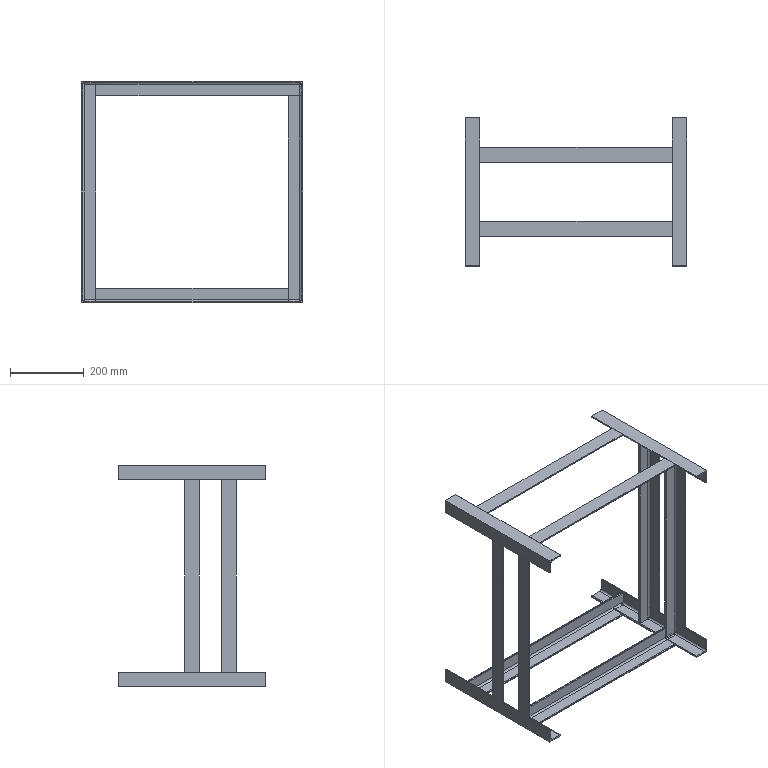Part | SolidWorks | features 3DProfileFeature 1, WeldMemberFeat 1, WeldmentFeature 1 | 12 solids | 184 faces | box 600 x 400 x 600 mm | volume 1841733 mm3 | plane 148 | cylinder 36 | commonest cylinder face diameters 2.667 x24 10 x12